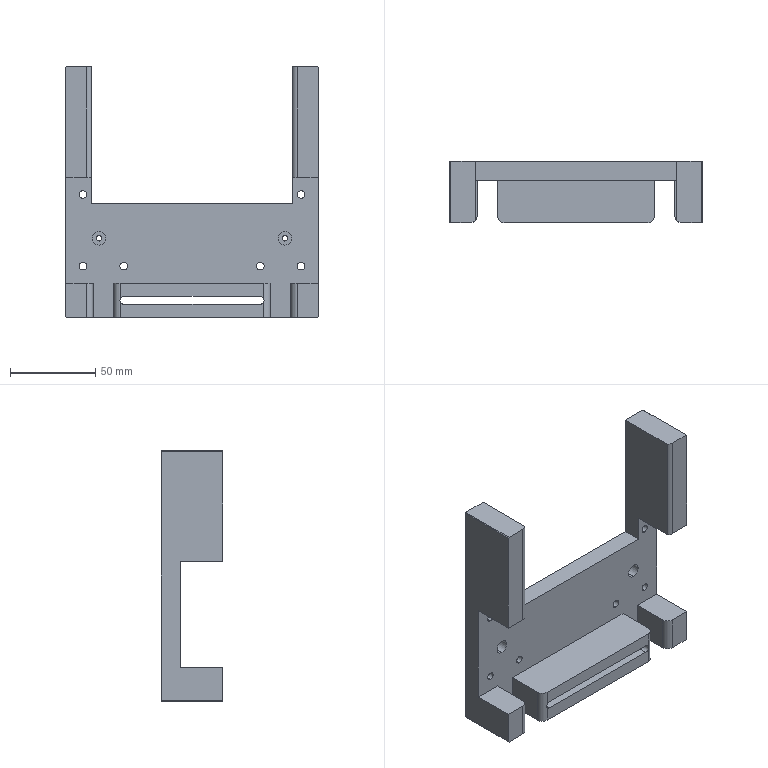Part | SolidWorks | features ICE 6, HoleWzd 2, Chamfer 1, Extrusion 1, Fillet 1 | 1 solid | 84 faces | box 148 x 36 x 147 mm | volume 224045 mm3 | cylinder 42 | plane 42 | commonest cylinder face diameters 8 x22 4.5 x14 3.3 x4 10.5 x2